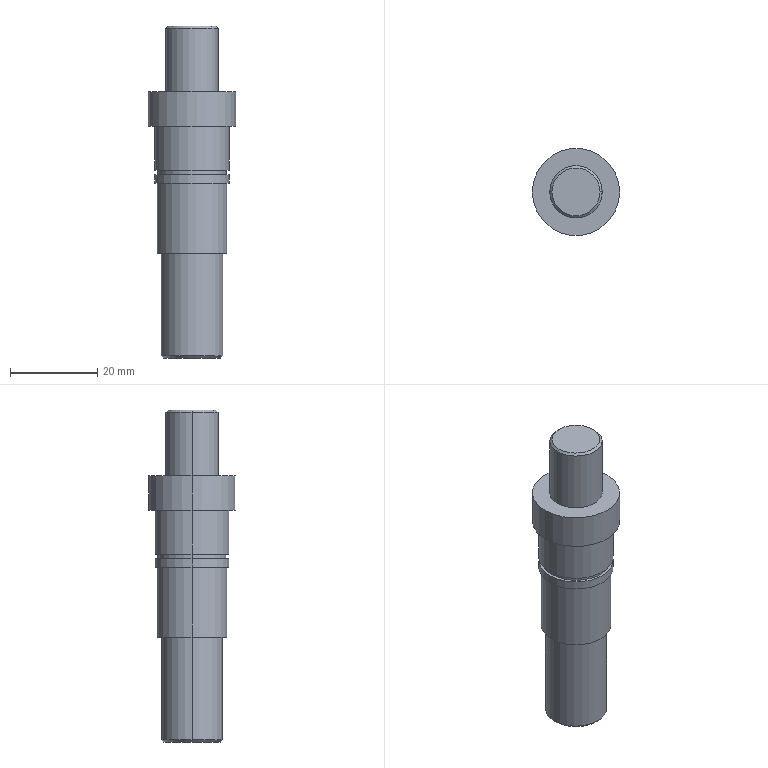Part | STEP file | 09-32 Fan blade connecting shaft | 1 solid | 26 faces | box 20 x 20 x 76 mm | volume 14029 mm3 | cylinder 14 | plane 8 | cone 4 | commonest cylinder face diameters 17 x4 12 x2 14 x2 15.7 x2 16 x2 20 x2